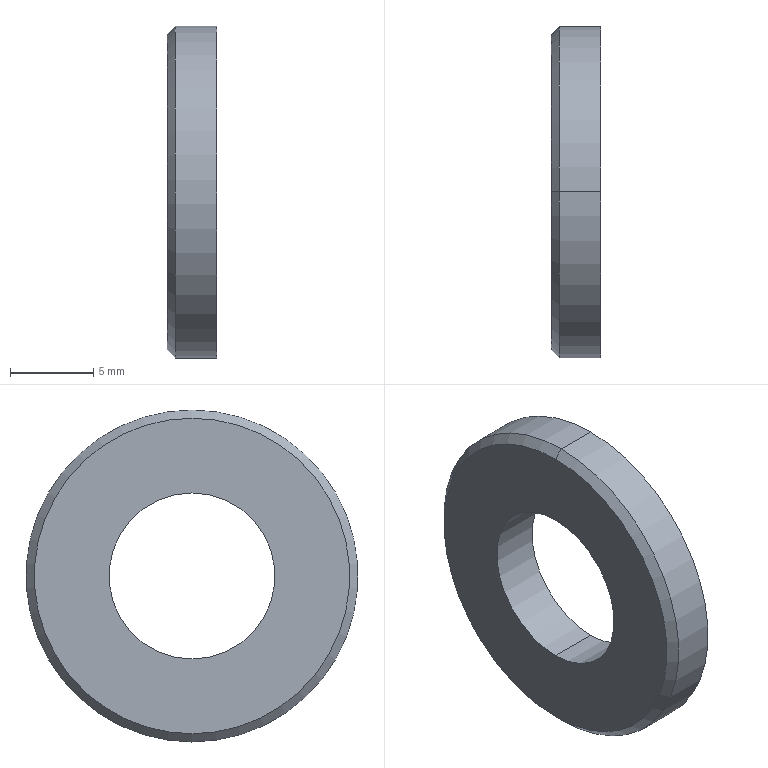Part | NX | features BREP 1 | 1 solid | 8 faces | box 3 x 20 x 20 mm | volume 699.135 mm3 | cylinder 4 | cone 2 | plane 2 | commonest cylinder face diameters 10 x2 20 x2
STEP:
#1=CARTESIAN_POINT('',(0.,0.,9.5));
#2=VERTEX_POINT('',#1);
#3=CARTESIAN_POINT('',(0.,0.,-9.5));
#4=VERTEX_POINT('',#3);
#5=CARTESIAN_POINT('',(0.,0.,0.));
#6=DIRECTION('',(-1.,0.,0.));
#7=DIRECTION('',(0.,0.,-1.));
#8=AXIS2_PLACEMENT_3D('',#5,#6,#7);
#9=CIRCLE('',#8,9.5);
#10=EDGE_CURVE('',#2,#4,#9,.T.);
#11=ORIENTED_EDGE('',*,*,#10,.F.);
#12=CARTESIAN_POINT('',(0.5,0.,10.));
#13=VERTEX_POINT('',#12);
#14=CARTESIAN_POINT('',(0.5,0.,10.));
#15=DIRECTION('',(0.7071,0.,0.7071));
#16=VECTOR('',#15,1000.);
#17=LINE('',#14,#16);
#18=EDGE_CURVE('',#13,#2,#17,.F.);
#19=ORIENTED_EDGE('',*,*,#18,.F.);
#20=CARTESIAN_POINT('',(0.5,0.,-10.));
#21=VERTEX_POINT('',#20);
#22=CARTESIAN_POINT('',(0.5,0.,0.));
#23=DIRECTION('',(1.,0.,0.));
#24=DIRECTION('',(0.,0.,-1.));
#25=AXIS2_PLACEMENT_3D('',#22,#23,#24);
#26=CIRCLE('',#25,10.);
#27=EDGE_CURVE('',#21,#13,#26,.T.);
#28=ORIENTED_EDGE('',*,*,#27,.F.);
#29=CARTESIAN_POINT('',(0.5,0.,-10.));
#30=DIRECTION('',(0.7071,0.,-0.7071));
#31=VECTOR('',#30,1000.);
#32=LINE('',#29,#31);
#33=EDGE_CURVE('',#21,#4,#32,.F.);
#34=ORIENTED_EDGE('',*,*,#33,.T.);
#35=EDGE_LOOP('',(#11,#19,#28,#34));
#36=FACE_BOUND('',#35,.T.);
#37=CARTESIAN_POINT('',(0.5,0.,0.));
#38=DIRECTION('',(1.,0.,0.));
#39=DIRECTION('',(0.,0.,1.));
#40=AXIS2_PLACEMENT_3D('',#37,#38,#39);
#41=CONICAL_SURFACE('',#40,10.,0.7854);
#42=ADVANCED_FACE('',(#36),#41,.T.);
#43=CARTESIAN_POINT('',(3.,0.,5.));
#44=VERTEX_POINT('',#43);
#45=CARTESIAN_POINT('',(3.,0.,-5.));
#46=VERTEX_POINT('',#45);
#47=CARTESIAN_POINT('',(3.,0.,0.));
#48=DIRECTION('',(1.,0.,0.));
#49=DIRECTION('',(0.,0.,-1.));
#50=AXIS2_PLACEMENT_3D('',#47,#48,#49);
#51=CIRCLE('',#50,5.);
#52=EDGE_CURVE('',#44,#46,#51,.T.);
#53=ORIENTED_EDGE('',*,*,#52,.T.);
#54=CARTESIAN_POINT('',(0.,0.,-5.));
#55=VERTEX_POINT('',#54);
#56=CARTESIAN_POINT('',(3.,0.,-5.));
#57=DIRECTION('',(-1.,0.,0.));
#58=VECTOR('',#57,1000.);
#59=LINE('',#56,#58);
#60=EDGE_CURVE('',#46,#55,#59,.T.);
#61=ORIENTED_EDGE('',*,*,#60,.T.);
#62=CARTESIAN_POINT('',(0.,0.,5.));
#63=VERTEX_POINT('',#62);
#64=CARTESIAN_POINT('',(0.,0.,0.));
#65=DIRECTION('',(1.,0.,0.));
#66=DIRECTION('',(0.,0.,-1.));
#67=AXIS2_PLACEMENT_3D('',#64,#65,#66);
#68=CIRCLE('',#67,5.);
#69=EDGE_CURVE('',#63,#55,#68,.T.);
#70=ORIENTED_EDGE('',*,*,#69,.F.);
#71=CARTESIAN_POINT('',(3.,0.,5.));
#72=DIRECTION('',(-1.,0.,0.));
#73=VECTOR('',#72,1000.);
#74=LINE('',#71,#73);
#75=EDGE_CURVE('',#44,#63,#74,.T.);
#76=ORIENTED_EDGE('',*,*,#75,.F.);
#77=EDGE_LOOP('',(#53,#61,#70,#76));
#78=FACE_BOUND('',#77,.T.);
#79=CARTESIAN_POINT('',(3.,0.,0.));
#80=DIRECTION('',(-1.,0.,0.));
#81=DIRECTION('',(0.,0.,-1.));
#82=AXIS2_PLACEMENT_3D('',#79,#80,#81);
#83=CYLINDRICAL_SURFACE('',#82,5.);
#84=ADVANCED_FACE('',(#78),#83,.F.);
#85=CARTESIAN_POINT('',(3.,0.,-10.));
#86=VERTEX_POINT('',#85);
#87=CARTESIAN_POINT('',(3.,0.,10.));
#88=VERTEX_POINT('',#87);
#89=CARTESIAN_POINT('',(3.,0.,0.));
#90=DIRECTION('',(1.,0.,0.));
#91=DIRECTION('',(0.,0.,-1.));
#92=AXIS2_PLACEMENT_3D('',#89,#90,#91);
#93=CIRCLE('',#92,10.);
#94=EDGE_CURVE('',#86,#88,#93,.T.);
#95=ORIENTED_EDGE('',*,*,#94,.F.);
#96=CARTESIAN_POINT('',(3.,0.,-10.));
#97=DIRECTION('',(-1.,0.,0.));
#98=VECTOR('',#97,1000.);
#99=LINE('',#96,#98);
#100=EDGE_CURVE('',#86,#21,#99,.T.);
#101=ORIENTED_EDGE('',*,*,#100,.T.);
#102=ORIENTED_EDGE('',*,*,#27,.T.);
#103=CARTESIAN_POINT('',(3.,0.,10.));
#104=DIRECTION('',(-1.,0.,0.));
#105=VECTOR('',#104,1000.);
#106=LINE('',#103,#105);
#107=EDGE_CURVE('',#88,#13,#106,.T.);
#108=ORIENTED_EDGE('',*,*,#107,.F.);
#109=EDGE_LOOP('',(#95,#101,#102,#108));
#110=FACE_BOUND('',#109,.T.);
#111=CARTESIAN_POINT('',(3.,0.,0.));
#112=DIRECTION('',(-1.,0.,0.));
#113=DIRECTION('',(0.,0.,-1.));
#114=AXIS2_PLACEMENT_3D('',#111,#112,#113);
#115=CYLINDRICAL_SURFACE('',#114,10.);
#116=ADVANCED_FACE('',(#110),#115,.T.);
#117=CARTESIAN_POINT('',(3.,0.,0.));
#118=DIRECTION('',(1.,0.,0.));
#119=DIRECTION('',(0.,0.,-1.));
#120=AXIS2_PLACEMENT_3D('',#117,#118,#119);
#121=CIRCLE('',#120,10.);
#122=EDGE_CURVE('',#88,#86,#121,.T.);
#123=ORIENTED_EDGE('',*,*,#122,.T.);
#124=ORIENTED_EDGE('',*,*,#94,.T.);
#125=EDGE_LOOP('',(#123,#124));
#126=FACE_BOUND('',#125,.T.);
#127=ORIENTED_EDGE('',*,*,#52,.F.);
#128=CARTESIAN_POINT('',(3.,0.,0.));
#129=DIRECTION('',(1.,0.,0.));
#130=DIRECTION('',(0.,0.,-1.));
#131=AXIS2_PLACEMENT_3D('',#128,#129,#130);
#132=CIRCLE('',#131,5.);
#133=EDGE_CURVE('',#46,#44,#132,.T.);
#134=ORIENTED_EDGE('',*,*,#133,.F.);
#135=EDGE_LOOP('',(#127,#134));
#136=FACE_BOUND('',#135,.T.);
#137=CARTESIAN_POINT('',(3.,0.,0.));
#138=DIRECTION('',(1.,0.,0.));
#139=DIRECTION('',(0.,0.,-1.));
#140=AXIS2_PLACEMENT_3D('',#137,#138,#139);
#141=PLANE('',#140);
#142=ADVANCED_FACE('',(#126,#136),#141,.T.);
#143=CARTESIAN_POINT('',(0.,0.,0.));
#144=DIRECTION('',(-1.,0.,0.));
#145=DIRECTION('',(0.,0.,-1.));
#146=AXIS2_PLACEMENT_3D('',#143,#144,#145);
#147=CIRCLE('',#146,9.5);
#148=EDGE_CURVE('',#4,#2,#147,.T.);
#149=ORIENTED_EDGE('',*,*,#148,.T.);
#150=ORIENTED_EDGE('',*,*,#10,.T.);
#151=EDGE_LOOP('',(#149,#150));
#152=FACE_BOUND('',#151,.T.);
#153=ORIENTED_EDGE('',*,*,#69,.T.);
#154=CARTESIAN_POINT('',(0.,0.,0.));
#155=DIRECTION('',(1.,0.,0.));
#156=DIRECTION('',(0.,0.,-1.));
#157=AXIS2_PLACEMENT_3D('',#154,#155,#156);
#158=CIRCLE('',#157,5.);
#159=EDGE_CURVE('',#55,#63,#158,.T.);
#160=ORIENTED_EDGE('',*,*,#159,.T.);
#161=EDGE_LOOP('',(#153,#160));
#162=FACE_BOUND('',#161,.T.);
#163=CARTESIAN_POINT('',(0.,0.,0.));
#164=DIRECTION('',(1.,0.,0.));
#165=DIRECTION('',(0.,0.,-1.));
#166=AXIS2_PLACEMENT_3D('',#163,#164,#165);
#167=PLANE('',#166);
#168=ADVANCED_FACE('',(#152,#162),#167,.F.);
#169=ORIENTED_EDGE('',*,*,#100,.F.);
#170=ORIENTED_EDGE('',*,*,#122,.F.);
#171=ORIENTED_EDGE('',*,*,#107,.T.);
#172=CARTESIAN_POINT('',(0.5,0.,0.));
#173=DIRECTION('',(1.,0.,0.));
#174=DIRECTION('',(0.,0.,-1.));
#175=AXIS2_PLACEMENT_3D('',#172,#173,#174);
#176=CIRCLE('',#175,10.);
#177=EDGE_CURVE('',#13,#21,#176,.T.);
#178=ORIENTED_EDGE('',*,*,#177,.T.);
#179=EDGE_LOOP('',(#169,#170,#171,#178));
#180=FACE_BOUND('',#179,.T.);
#181=CARTESIAN_POINT('',(3.,0.,0.));
#182=DIRECTION('',(-1.,0.,0.));
#183=DIRECTION('',(0.,0.,-1.));
#184=AXIS2_PLACEMENT_3D('',#181,#182,#183);
#185=CYLINDRICAL_SURFACE('',#184,10.);
#186=ADVANCED_FACE('',(#180),#185,.T.);
#187=ORIENTED_EDGE('',*,*,#60,.F.);
#188=ORIENTED_EDGE('',*,*,#133,.T.);
#189=ORIENTED_EDGE('',*,*,#75,.T.);
#190=ORIENTED_EDGE('',*,*,#159,.F.);
#191=EDGE_LOOP('',(#187,#188,#189,#190));
#192=FACE_BOUND('',#191,.T.);
#193=CARTESIAN_POINT('',(3.,0.,0.));
#194=DIRECTION('',(-1.,0.,0.));
#195=DIRECTION('',(0.,0.,-1.));
#196=AXIS2_PLACEMENT_3D('',#193,#194,#195);
#197=CYLINDRICAL_SURFACE('',#196,5.);
#198=ADVANCED_FACE('',(#192),#197,.F.);
#199=ORIENTED_EDGE('',*,*,#18,.T.);
#200=ORIENTED_EDGE('',*,*,#148,.F.);
#201=ORIENTED_EDGE('',*,*,#33,.F.);
#202=ORIENTED_EDGE('',*,*,#177,.F.);
#203=EDGE_LOOP('',(#199,#200,#201,#202));
#204=FACE_BOUND('',#203,.T.);
#205=CARTESIAN_POINT('',(0.5,0.,0.));
#206=DIRECTION('',(1.,0.,0.));
#207=DIRECTION('',(0.,0.,1.));
#208=AXIS2_PLACEMENT_3D('',#205,#206,#207);
#209=CONICAL_SURFACE('',#208,10.,0.7854);
#210=ADVANCED_FACE('',(#204),#209,.T.);
#211=CLOSED_SHELL('',(#42,#84,#116,#142,#168,#186,#198,#210));
#212=MANIFOLD_SOLID_BREP('',#211);
#213=(LENGTH_UNIT()NAMED_UNIT(*)SI_UNIT(.MILLI.,.METRE.));
#214=UNCERTAINTY_MEASURE_WITH_UNIT(LENGTH_MEASURE(0.00001),#213,'','');
#215=(NAMED_UNIT(*)PLANE_ANGLE_UNIT()SI_UNIT($,.RADIAN.));
#216=(NAMED_UNIT(*)SI_UNIT($,.STERADIAN.)SOLID_ANGLE_UNIT());
#217=(GEOMETRIC_REPRESENTATION_CONTEXT(3)GLOBAL_UNCERTAINTY_ASSIGNED_CONTEXT((#214))GLOBAL_UNIT_ASSIGNED_CONTEXT((#213,#215,#216))REPRESENTATION_CONTEXT('',''));
#218=ADVANCED_BREP_SHAPE_REPRESENTATION('',(#212),#217);